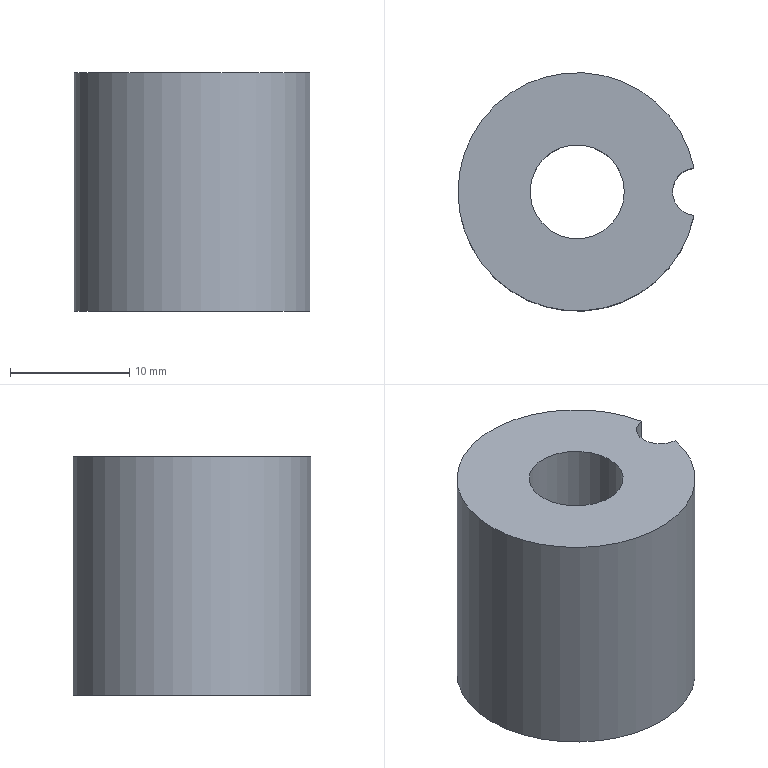Part | NX | features solid 2 | 1 solid | 7 faces | box 19.8 x 20 x 20 mm | volume 4274 mm3 | cylinder 4 | plane 3 | commonest cylinder face diameters 4 x1 7.9 x1 12.6 x1 20 x1
STEP:
#1=CARTESIAN_POINT('',(409.8,-327.519,-13.));
#2=VERTEX_POINT('',#1);
#3=CARTESIAN_POINT('',(409.8,-327.519,7.));
#4=VERTEX_POINT('',#3);
#5=CARTESIAN_POINT('',(409.8,-327.519,-3.));
#6=DIRECTION('',(0.,0.,1.));
#7=VECTOR('',#6,1000.);
#8=LINE('',#5,#7);
#9=EDGE_CURVE('',#2,#4,#8,.T.);
#10=ORIENTED_EDGE('',*,*,#9,.F.);
#11=CARTESIAN_POINT('',(409.8,-331.499,-13.));
#12=VERTEX_POINT('',#11);
#13=CARTESIAN_POINT('',(400.,-329.509,-13.));
#14=DIRECTION('',(0.,0.,1.));
#15=DIRECTION('',(1.,0.,0.));
#16=AXIS2_PLACEMENT_3D('',#13,#14,#15);
#17=CIRCLE('',#16,10.);
#18=EDGE_CURVE('',#2,#12,#17,.T.);
#19=ORIENTED_EDGE('',*,*,#18,.T.);
#20=CARTESIAN_POINT('',(409.8,-331.499,7.));
#21=VERTEX_POINT('',#20);
#22=CARTESIAN_POINT('',(409.8,-331.499,-3.));
#23=DIRECTION('',(0.,0.,1.));
#24=VECTOR('',#23,1000.);
#25=LINE('',#22,#24);
#26=EDGE_CURVE('',#21,#12,#25,.F.);
#27=ORIENTED_EDGE('',*,*,#26,.F.);
#28=CARTESIAN_POINT('',(400.,-329.509,7.));
#29=DIRECTION('',(0.,0.,1.));
#30=DIRECTION('',(1.,0.,0.));
#31=AXIS2_PLACEMENT_3D('',#28,#29,#30);
#32=CIRCLE('',#31,10.);
#33=EDGE_CURVE('',#4,#21,#32,.T.);
#34=ORIENTED_EDGE('',*,*,#33,.F.);
#35=EDGE_LOOP('',(#10,#19,#27,#34));
#36=FACE_BOUND('',#35,.T.);
#37=CARTESIAN_POINT('',(400.,-329.509,-13.));
#38=DIRECTION('',(0.,0.,1.));
#39=DIRECTION('',(1.,0.,0.));
#40=AXIS2_PLACEMENT_3D('',#37,#38,#39);
#41=CYLINDRICAL_SURFACE('',#40,10.);
#42=ADVANCED_FACE('',(#36),#41,.T.);
#43=CARTESIAN_POINT('',(406.3,-329.509,-13.));
#44=VERTEX_POINT('',#43);
#45=CARTESIAN_POINT('',(400.,-329.509,-13.));
#46=DIRECTION('',(0.,0.,1.));
#47=DIRECTION('',(1.,0.,0.));
#48=AXIS2_PLACEMENT_3D('',#45,#46,#47);
#49=CIRCLE('',#48,6.3);
#50=EDGE_CURVE('',#44,#44,#49,.T.);
#51=ORIENTED_EDGE('',*,*,#50,.T.);
#52=EDGE_LOOP('',(#51));
#53=FACE_BOUND('',#52,.T.);
#54=ORIENTED_EDGE('',*,*,#18,.F.);
#55=CARTESIAN_POINT('',(410.,-329.509,-13.));
#56=DIRECTION('',(0.,0.,1.));
#57=DIRECTION('',(1.,0.,0.));
#58=AXIS2_PLACEMENT_3D('',#55,#56,#57);
#59=CIRCLE('',#58,2.);
#60=EDGE_CURVE('',#2,#12,#59,.T.);
#61=ORIENTED_EDGE('',*,*,#60,.T.);
#62=EDGE_LOOP('',(#54,#61));
#63=FACE_BOUND('',#62,.T.);
#64=CARTESIAN_POINT('',(400.,-329.509,-13.));
#65=DIRECTION('',(0.,0.,1.));
#66=DIRECTION('',(1.,0.,0.));
#67=AXIS2_PLACEMENT_3D('',#64,#65,#66);
#68=PLANE('',#67);
#69=ADVANCED_FACE('',(#53,#63),#68,.F.);
#70=CARTESIAN_POINT('',(403.95,-329.509,7.));
#71=VERTEX_POINT('',#70);
#72=CARTESIAN_POINT('',(400.,-329.509,7.));
#73=DIRECTION('',(0.,0.,1.));
#74=DIRECTION('',(1.,0.,0.));
#75=AXIS2_PLACEMENT_3D('',#72,#73,#74);
#76=CIRCLE('',#75,3.95);
#77=EDGE_CURVE('',#71,#71,#76,.T.);
#78=ORIENTED_EDGE('',*,*,#77,.F.);
#79=EDGE_LOOP('',(#78));
#80=FACE_BOUND('',#79,.T.);
#81=CARTESIAN_POINT('',(410.,-329.509,7.));
#82=DIRECTION('',(0.,0.,1.));
#83=DIRECTION('',(1.,0.,0.));
#84=AXIS2_PLACEMENT_3D('',#81,#82,#83);
#85=CIRCLE('',#84,2.);
#86=EDGE_CURVE('',#4,#21,#85,.T.);
#87=ORIENTED_EDGE('',*,*,#86,.F.);
#88=ORIENTED_EDGE('',*,*,#33,.T.);
#89=EDGE_LOOP('',(#87,#88));
#90=FACE_BOUND('',#89,.T.);
#91=CARTESIAN_POINT('',(400.,-329.509,7.));
#92=DIRECTION('',(0.,0.,1.));
#93=DIRECTION('',(1.,0.,0.));
#94=AXIS2_PLACEMENT_3D('',#91,#92,#93);
#95=PLANE('',#94);
#96=ADVANCED_FACE('',(#80,#90),#95,.T.);
#97=ORIENTED_EDGE('',*,*,#50,.F.);
#98=EDGE_LOOP('',(#97));
#99=FACE_BOUND('',#98,.T.);
#100=CARTESIAN_POINT('',(406.3,-329.509,-1.));
#101=VERTEX_POINT('',#100);
#102=CARTESIAN_POINT('',(400.,-329.509,-1.));
#103=DIRECTION('',(0.,0.,1.));
#104=DIRECTION('',(1.,0.,0.));
#105=AXIS2_PLACEMENT_3D('',#102,#103,#104);
#106=CIRCLE('',#105,6.3);
#107=EDGE_CURVE('',#101,#101,#106,.T.);
#108=ORIENTED_EDGE('',*,*,#107,.T.);
#109=EDGE_LOOP('',(#108));
#110=FACE_BOUND('',#109,.T.);
#111=CARTESIAN_POINT('',(400.,-329.509,-13.));
#112=DIRECTION('',(0.,0.,1.));
#113=DIRECTION('',(1.,0.,0.));
#114=AXIS2_PLACEMENT_3D('',#111,#112,#113);
#115=CYLINDRICAL_SURFACE('',#114,6.3);
#116=ADVANCED_FACE('',(#99,#110),#115,.F.);
#117=CARTESIAN_POINT('',(403.95,-329.509,-1.));
#118=VERTEX_POINT('',#117);
#119=CARTESIAN_POINT('',(400.,-329.509,-1.));
#120=DIRECTION('',(0.,0.,1.));
#121=DIRECTION('',(1.,0.,0.));
#122=AXIS2_PLACEMENT_3D('',#119,#120,#121);
#123=CIRCLE('',#122,3.95);
#124=EDGE_CURVE('',#118,#118,#123,.T.);
#125=ORIENTED_EDGE('',*,*,#124,.T.);
#126=EDGE_LOOP('',(#125));
#127=FACE_BOUND('',#126,.T.);
#128=ORIENTED_EDGE('',*,*,#107,.F.);
#129=EDGE_LOOP('',(#128));
#130=FACE_BOUND('',#129,.T.);
#131=CARTESIAN_POINT('',(400.,-329.509,-1.));
#132=DIRECTION('',(0.,0.,1.));
#133=DIRECTION('',(1.,0.,0.));
#134=AXIS2_PLACEMENT_3D('',#131,#132,#133);
#135=PLANE('',#134);
#136=ADVANCED_FACE('',(#127,#130),#135,.F.);
#137=ORIENTED_EDGE('',*,*,#9,.T.);
#138=ORIENTED_EDGE('',*,*,#86,.T.);
#139=ORIENTED_EDGE('',*,*,#26,.T.);
#140=ORIENTED_EDGE('',*,*,#60,.F.);
#141=EDGE_LOOP('',(#137,#138,#139,#140));
#142=FACE_BOUND('',#141,.T.);
#143=CARTESIAN_POINT('',(410.,-329.509,-13.));
#144=DIRECTION('',(0.,0.,1.));
#145=DIRECTION('',(1.,0.,0.));
#146=AXIS2_PLACEMENT_3D('',#143,#144,#145);
#147=CYLINDRICAL_SURFACE('',#146,2.);
#148=ADVANCED_FACE('',(#142),#147,.F.);
#149=ORIENTED_EDGE('',*,*,#77,.T.);
#150=EDGE_LOOP('',(#149));
#151=FACE_BOUND('',#150,.T.);
#152=ORIENTED_EDGE('',*,*,#124,.F.);
#153=EDGE_LOOP('',(#152));
#154=FACE_BOUND('',#153,.T.);
#155=CARTESIAN_POINT('',(400.,-329.509,-13.));
#156=DIRECTION('',(0.,0.,1.));
#157=DIRECTION('',(1.,0.,0.));
#158=AXIS2_PLACEMENT_3D('',#155,#156,#157);
#159=CYLINDRICAL_SURFACE('',#158,3.95);
#160=ADVANCED_FACE('',(#151,#154),#159,.F.);
#161=CLOSED_SHELL('',(#42,#69,#96,#116,#136,#148,#160));
#162=MANIFOLD_SOLID_BREP('',#161);
#163=(LENGTH_UNIT()NAMED_UNIT(*)SI_UNIT(.MILLI.,.METRE.));
#164=UNCERTAINTY_MEASURE_WITH_UNIT(LENGTH_MEASURE(0.00001),#163,'','');
#165=(NAMED_UNIT(*)PLANE_ANGLE_UNIT()SI_UNIT($,.RADIAN.));
#166=(NAMED_UNIT(*)SI_UNIT($,.STERADIAN.)SOLID_ANGLE_UNIT());
#167=(GEOMETRIC_REPRESENTATION_CONTEXT(3)GLOBAL_UNCERTAINTY_ASSIGNED_CONTEXT((#164))GLOBAL_UNIT_ASSIGNED_CONTEXT((#163,#165,#166))REPRESENTATION_CONTEXT('',''));
#168=ADVANCED_BREP_SHAPE_REPRESENTATION('',(#162),#167);